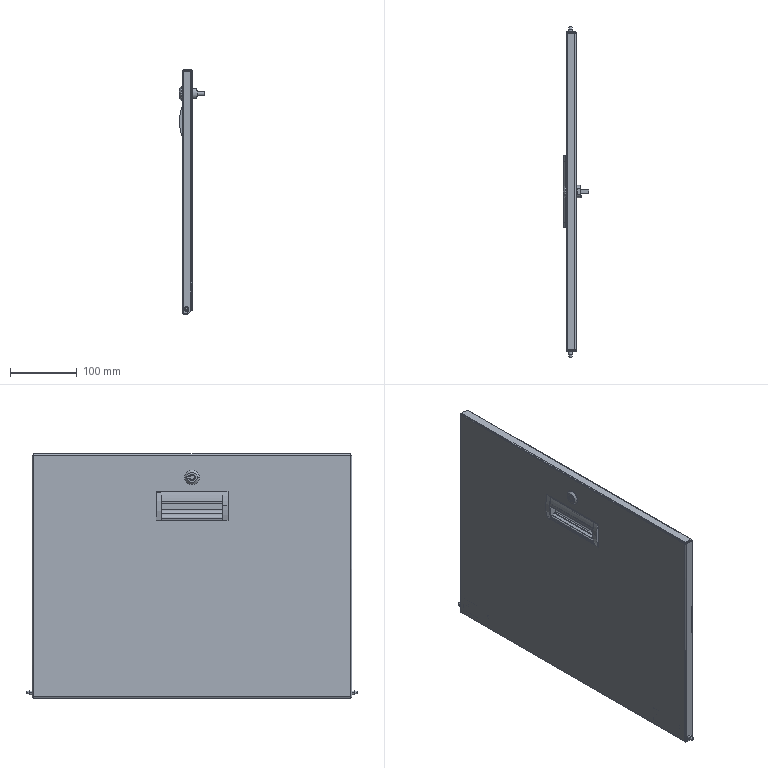Part | SolidWorks | 9 solids | 275 faces | box 37.5 x 494 x 364.5 mm | volume 343141 mm3 | plane 151 | cylinder 106 | spline 8 | cone 6 | torus 4 | commonest cylinder face diameters 1 x18 7 x10 5.5 x8 6 x8 0.6 x7 3.6 x7